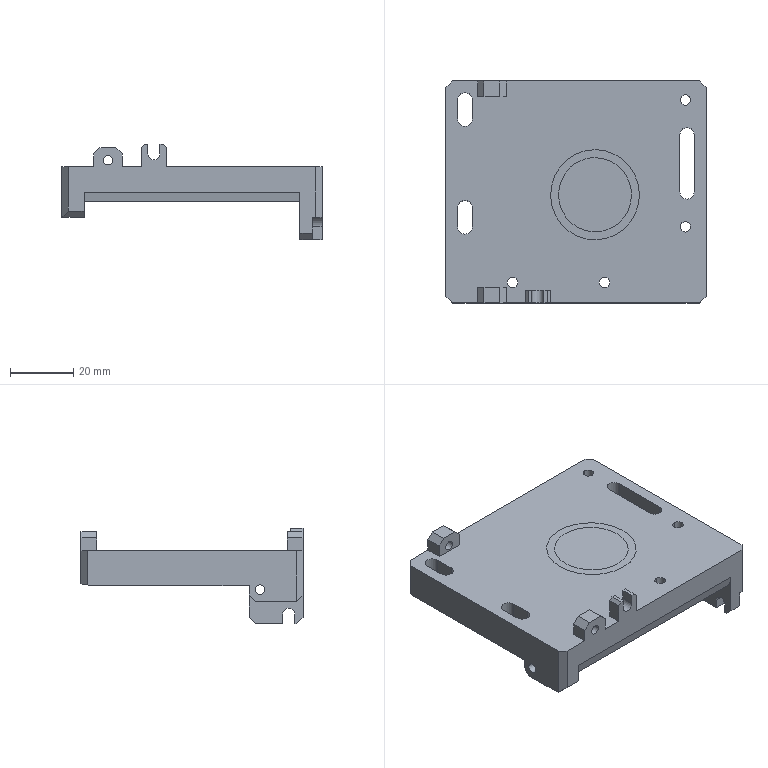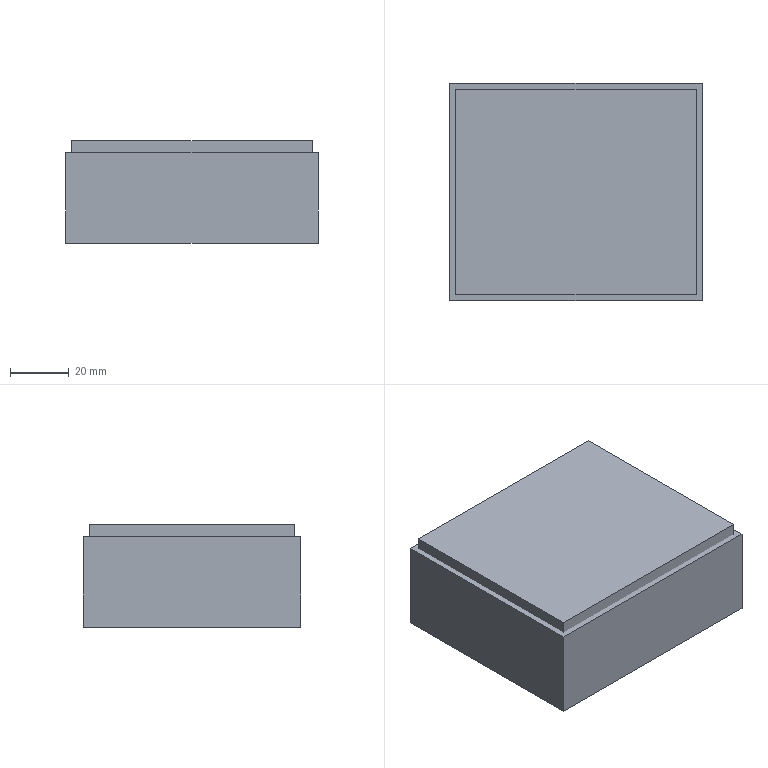CAM job | NX | 3+2 milling, drilling | part box 82 x 70 x 30 mm | stock box 86 x 74 x 35 mm
Tools:
number,name,description,diameter,corner_radius,flute_length,length,flutes
10,D10,Milling Tool-5 Parameters,10.0,0.0,50.0,75.0,2
11,D10JING,Milling Tool-5 Parameters,10.0,0.0,50.0,75.0,2
4,D4,Milling Tool-5 Parameters,4.0,0.0,50.0,75.0,2
3,D3,Milling Tool-5 Parameters,3.0,0.0,50.0,75.0,2
14,D1.5,Milling Tool-5 Parameters,1.5,0.0,50.0,75.0,2
12,R0.75,Milling Tool-5 Parameters,1.5,0.75,50.0,75.0,2
5,D3R0.5,Milling Tool-5 Parameters,3.0,0.5,50.0,75.0,2
7,D6A45,Milling Tool-5 Parameters,6.0,0.0,50.0,75.0,2
13,3.3ZT,Drilling Tool,3.3,0.0,35.0,50.0,2
8,T6H1,Milling Tool-T Cutter,6.0,,1.0,25.0,4
9,D2.4XYD,Thread Mill,2.4,0.0,0.5,50.0,2
Operations:
program,operation,operation_type,tool,method,geometry_group,spindle_rpm,surface_speed,feed_per_tooth,feed_cut,feed_plunge,cut_length_mm,path_length_mm,cut_time_min,machine_time_min
1,FLOOR_WALL,VolumeBased25DMillingOperation,D10JING,METHOD,A,9500.0,298.0,0.0658,1250.0,100.0,1605.997,1659.997,1.285,1.29
1,ZLEVEL_PROFILE,ZLevelMilling,D10,METHOD,A,9500.0,298.0,0.1579,3000.0,1000.0,19950.094,20037.094,6.676,6.684
1,CAVITY_MILL,CavityMilling,D10,METHOD,A,9500.0,298.0,0.1579,3000.0,1000.0,32479.726,33004.007,11.613,11.665
1,FLOOR_WALL_1,VolumeBased25DMillingOperation,D10JING,METHOD,A,9500.0,298.0,0.0658,1250.0,100.0,1647.553,2212.329,1.318,1.375
1,ZLEVEL_PROFILE_COPY,ZLevelMilling,D10JING,METHOD,A,9500.0,298.0,0.0632,1200.0,1000.0,678.136,885.496,0.5665,0.5872
1,ZLEVEL_PROFILE_COPY_1,ZLevelMilling,D4,METHOD,A,9500.0,119.0,0.0789,1500.0,1000.0,2559.356,3032.051,1.741,1.788
1,ZLEVEL_PROFILE_COPY_1_COPY,ZLevelMilling,D3,METHOD,A,9500.0,89.0,0.0632,1200.0,1000.0,438.069,520.769,0.3704,0.3786
1,CAVITY_MILL_COPY,CavityMilling,D3,METHOD,A,9500.0,89.0,0.0579,1100.0,1000.0,906.472,1180.293,0.834,0.8614
1,CAVITY_MILL_COPY_COPY,CavityMilling,D1.5,METHOD,A,9500.0,44.0,0.0579,1100.0,1000.0,614.344,1048.651,0.575,0.6184
1,CAVITY_MILL_COPY_COPY_COPY,CavityMilling,D1.5,METHOD,A,9500.0,44.0,0.0579,1100.0,1000.0,137.088,1860.447,0.1293,0.3017
1,FIXED_CONTOUR,SurfaceContour,R0.75,METHOD,A,9500.0,44.0,0.1053,2000.0,1000.0,614.724,729.785,0.3152,0.3267
1,FIXED_CONTOUR_COPY,SurfaceContour,D3R0.5,METHOD,A,9500.0,44.0,0.1053,2000.0,1000.0,5012.261,5090.261,2.508,2.516
1,ZLEVEL_PROFILE_1,ZLevelMilling,D3R0.5,METHOD,A,9500.0,89.0,0.1316,2500.0,1000.0,535.813,701.833,0.2171,0.2337
1,ZLEVEL_PROFILE_1_COPY,ZLevelMilling,D3R0.5,METHOD,A,9500.0,89.0,0.1316,2500.0,1000.0,466.749,605.014,0.1894,0.2033
1,ZLEVEL_PROFILE_1_COPY_COPY,ZLevelMilling,D3R0.5,METHOD,A,9500.0,89.0,0.1316,2500.0,1000.0,2399.799,2484.398,0.9613,0.9698
1,DRILLING,Operation,D6A45,METHOD,A,5000.0,94.0,0.025,250.0,0.0,20.1,233.54,0.0804,0.1017
1,PLANAR_MILL,PlanarMilling,D6A45,METHOD,A,9500.0,179.0,0.0658,1250.0,100.0,215.285,747.494,0.1722,0.2254
1,PLANAR_MILL_COPY,PlanarMilling,D6A45,METHOD,A,9500.0,179.0,0.0658,1250.0,100.0,58.291,131.291,0.0466,0.0539
1,PLANAR_MILL_COPY_COPY,PlanarMilling,D6A45,METHOD,A,9500.0,179.0,0.0658,1250.0,100.0,46.165,105.165,0.0369,0.0428
1,DRILLING_COPY,Operation,3.3ZT,METHOD,A,2000.0,20.0,0.0375,150.0,0.0,65.966,325.271,0.4398,0.4657
2,FLOOR_WALL_COPY,VolumeBased25DMillingOperation,D10JING,METHOD,B,9500.0,298.0,0.0658,1250.0,100.0,14559.969,16140.49,11.648,11.806
2,CAVITY_MILL_COPY_1,CavityMilling,D10,METHOD,B,9500.0,298.0,0.1579,3000.0,1000.0,17203.835,17613.566,6.16,6.201
2,CAVITY_MILL_COPY_COPY_1,CavityMilling,D4,METHOD,B,9500.0,89.0,0.0579,1100.0,1000.0,1006.004,1398.0,0.9294,0.9686
2,FLOOR_WALL_1_COPY,VolumeBased25DMillingOperation,D4,METHOD,B,9500.0,119.0,0.0658,1250.0,100.0,3440.679,4072.497,2.752,2.82
2,CAVITY_MILL_COPY_COPY_2,CavityMilling,D3,METHOD,B,9500.0,89.0,0.0579,1100.0,1000.0,462.759,643.236,0.4281,0.4461
2,CAVITY_MILL_COPY_COPY_COPY_COPY,CavityMilling,D1.5,METHOD,B,9500.0,44.0,0.0579,1100.0,1000.0,148.767,294.548,0.1372,0.1517
2,FIXED_CONTOUR_COPY_1,SurfaceContour,R0.75,METHOD,B,9500.0,44.0,0.1053,2000.0,1000.0,427.57,481.57,0.2173,0.2227
2,ZLEVEL_PROFILE_1_COPY_1,ZLevelMilling,D3R0.5,METHOD,B,9500.0,89.0,0.1316,2500.0,1000.0,220.508,348.527,0.0909,0.1037
2,ZLEVEL_PROFILE_1_COPY_1_COPY,ZLevelMilling,D3R0.5,METHOD,B,9500.0,89.0,0.1316,2500.0,1000.0,863.629,1197.554,0.3509,0.3843
2,PLANAR_MILL_COPY_COPY_COPY,PlanarMilling,D6A45,METHOD,B,9500.0,179.0,0.0658,1250.0,100.0,416.135,1163.131,0.3329,0.4076
3,HOLE_MILLING,CylinderMilling,D10,METHOD,C,9500.0,298.0,0.0789,1500.0,100.0,1791.401,1915.431,1.194,1.207
3,HOLE_MILLING_COPY,CylinderMilling,D10,METHOD,C,9500.0,298.0,0.0789,1500.0,100.0,459.498,586.528,0.3063,0.319
3,HOLE_MILLING_COPY_COPY,CylinderMilling,D10,METHOD,C,9500.0,298.0,0.0789,1500.0,100.0,956.478,1095.619,0.6377,0.6516
3,PLANAR_MILL_1,PlanarMilling,T6H1,METHOD,C,8000.0,201.0,0.0391,1250.0,100.0,743.585,861.615,0.5949,0.6067
3,THREAD_MILLING,ThreadMilling,D2.4XYD,METHOD,C,7500.0,56.0,0.0833,1250.0,100.0,4446.838,4578.008,3.558,3.571